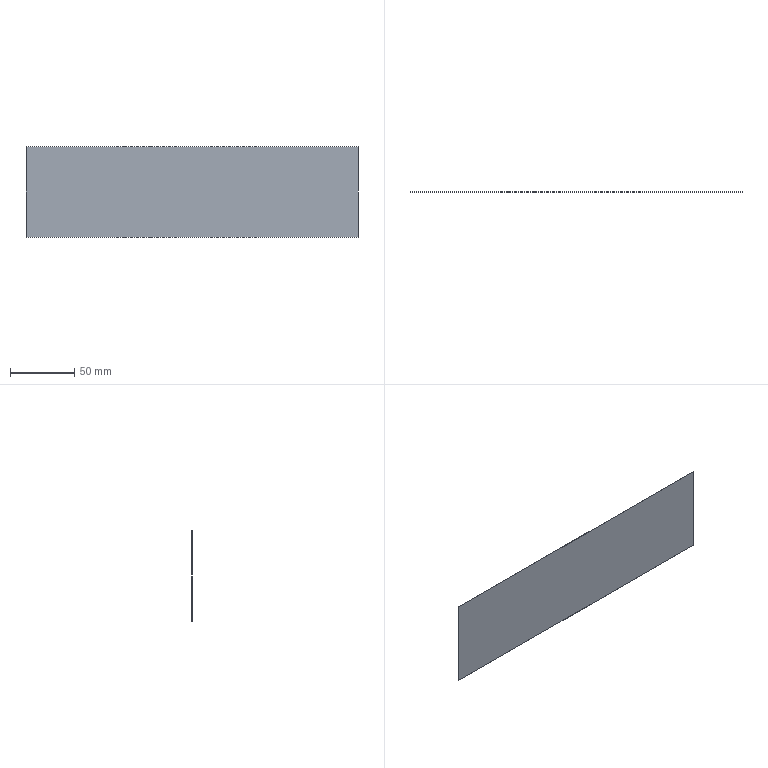Part | NX | features BREP 1 | 1 solid | 6 faces | box 258 x 0.1 x 70 mm | volume 1806 mm3 | plane 6
STEP:
#1=CARTESIAN_POINT('',(129.,0.,35.));
#2=VERTEX_POINT('',#1);
#3=CARTESIAN_POINT('',(129.,0.,-35.));
#4=VERTEX_POINT('',#3);
#5=CARTESIAN_POINT('',(129.,0.,-35.));
#6=DIRECTION('',(0.,0.,-1.));
#7=VECTOR('',#6,1000.);
#8=LINE('',#5,#7);
#9=EDGE_CURVE('',#2,#4,#8,.T.);
#10=ORIENTED_EDGE('',*,*,#9,.F.);
#11=CARTESIAN_POINT('',(-129.,0.,35.));
#12=VERTEX_POINT('',#11);
#13=CARTESIAN_POINT('',(-129.,0.,35.));
#14=DIRECTION('',(1.,0.,0.));
#15=VECTOR('',#14,1000.);
#16=LINE('',#13,#15);
#17=EDGE_CURVE('',#12,#2,#16,.T.);
#18=ORIENTED_EDGE('',*,*,#17,.F.);
#19=CARTESIAN_POINT('',(-129.,0.,-35.));
#20=VERTEX_POINT('',#19);
#21=CARTESIAN_POINT('',(-129.,0.,-35.));
#22=DIRECTION('',(0.,0.,1.));
#23=VECTOR('',#22,1000.);
#24=LINE('',#21,#23);
#25=EDGE_CURVE('',#20,#12,#24,.T.);
#26=ORIENTED_EDGE('',*,*,#25,.F.);
#27=CARTESIAN_POINT('',(-129.,0.,-35.));
#28=DIRECTION('',(-1.,0.,0.));
#29=VECTOR('',#28,1000.);
#30=LINE('',#27,#29);
#31=EDGE_CURVE('',#4,#20,#30,.T.);
#32=ORIENTED_EDGE('',*,*,#31,.F.);
#33=EDGE_LOOP('',(#10,#18,#26,#32));
#34=FACE_BOUND('',#33,.T.);
#35=CARTESIAN_POINT('',(0.,0.,0.));
#36=DIRECTION('',(0.,1.,0.));
#37=DIRECTION('',(0.,0.,1.));
#38=AXIS2_PLACEMENT_3D('',#35,#36,#37);
#39=PLANE('',#38);
#40=ADVANCED_FACE('',(#34),#39,.F.);
#41=CARTESIAN_POINT('',(129.,0.1,35.));
#42=VERTEX_POINT('',#41);
#43=CARTESIAN_POINT('',(129.,0.1,-35.));
#44=VERTEX_POINT('',#43);
#45=CARTESIAN_POINT('',(129.,0.1,-35.));
#46=DIRECTION('',(0.,0.,-1.));
#47=VECTOR('',#46,1000.);
#48=LINE('',#45,#47);
#49=EDGE_CURVE('',#42,#44,#48,.T.);
#50=ORIENTED_EDGE('',*,*,#49,.T.);
#51=CARTESIAN_POINT('',(-129.,0.1,-35.));
#52=VERTEX_POINT('',#51);
#53=CARTESIAN_POINT('',(-129.,0.1,-35.));
#54=DIRECTION('',(-1.,0.,0.));
#55=VECTOR('',#54,1000.);
#56=LINE('',#53,#55);
#57=EDGE_CURVE('',#44,#52,#56,.T.);
#58=ORIENTED_EDGE('',*,*,#57,.T.);
#59=CARTESIAN_POINT('',(-129.,0.1,35.));
#60=VERTEX_POINT('',#59);
#61=CARTESIAN_POINT('',(-129.,0.1,-35.));
#62=DIRECTION('',(0.,0.,1.));
#63=VECTOR('',#62,1000.);
#64=LINE('',#61,#63);
#65=EDGE_CURVE('',#52,#60,#64,.T.);
#66=ORIENTED_EDGE('',*,*,#65,.T.);
#67=CARTESIAN_POINT('',(-129.,0.1,35.));
#68=DIRECTION('',(1.,0.,0.));
#69=VECTOR('',#68,1000.);
#70=LINE('',#67,#69);
#71=EDGE_CURVE('',#60,#42,#70,.T.);
#72=ORIENTED_EDGE('',*,*,#71,.T.);
#73=EDGE_LOOP('',(#50,#58,#66,#72));
#74=FACE_BOUND('',#73,.T.);
#75=CARTESIAN_POINT('',(0.,0.1,0.));
#76=DIRECTION('',(0.,1.,0.));
#77=DIRECTION('',(0.,0.,1.));
#78=AXIS2_PLACEMENT_3D('',#75,#76,#77);
#79=PLANE('',#78);
#80=ADVANCED_FACE('',(#74),#79,.T.);
#81=ORIENTED_EDGE('',*,*,#17,.T.);
#82=CARTESIAN_POINT('',(129.,0.1,35.));
#83=DIRECTION('',(0.,-1.,0.));
#84=VECTOR('',#83,1000.);
#85=LINE('',#82,#84);
#86=EDGE_CURVE('',#42,#2,#85,.T.);
#87=ORIENTED_EDGE('',*,*,#86,.F.);
#88=ORIENTED_EDGE('',*,*,#71,.F.);
#89=CARTESIAN_POINT('',(-129.,0.1,35.));
#90=DIRECTION('',(0.,-1.,0.));
#91=VECTOR('',#90,1000.);
#92=LINE('',#89,#91);
#93=EDGE_CURVE('',#60,#12,#92,.T.);
#94=ORIENTED_EDGE('',*,*,#93,.T.);
#95=EDGE_LOOP('',(#81,#87,#88,#94));
#96=FACE_BOUND('',#95,.T.);
#97=CARTESIAN_POINT('',(-129.,0.1,35.));
#98=DIRECTION('',(0.,0.,-1.));
#99=DIRECTION('',(-1.,0.,0.));
#100=AXIS2_PLACEMENT_3D('',#97,#98,#99);
#101=PLANE('',#100);
#102=ADVANCED_FACE('',(#96),#101,.F.);
#103=ORIENTED_EDGE('',*,*,#25,.T.);
#104=ORIENTED_EDGE('',*,*,#93,.F.);
#105=ORIENTED_EDGE('',*,*,#65,.F.);
#106=CARTESIAN_POINT('',(-129.,0.1,-35.));
#107=DIRECTION('',(0.,-1.,0.));
#108=VECTOR('',#107,1000.);
#109=LINE('',#106,#108);
#110=EDGE_CURVE('',#52,#20,#109,.T.);
#111=ORIENTED_EDGE('',*,*,#110,.T.);
#112=EDGE_LOOP('',(#103,#104,#105,#111));
#113=FACE_BOUND('',#112,.T.);
#114=CARTESIAN_POINT('',(-129.,0.1,-35.));
#115=DIRECTION('',(1.,0.,0.));
#116=DIRECTION('',(0.,0.,-1.));
#117=AXIS2_PLACEMENT_3D('',#114,#115,#116);
#118=PLANE('',#117);
#119=ADVANCED_FACE('',(#113),#118,.F.);
#120=ORIENTED_EDGE('',*,*,#31,.T.);
#121=ORIENTED_EDGE('',*,*,#110,.F.);
#122=ORIENTED_EDGE('',*,*,#57,.F.);
#123=CARTESIAN_POINT('',(129.,0.1,-35.));
#124=DIRECTION('',(0.,-1.,0.));
#125=VECTOR('',#124,1000.);
#126=LINE('',#123,#125);
#127=EDGE_CURVE('',#44,#4,#126,.T.);
#128=ORIENTED_EDGE('',*,*,#127,.T.);
#129=EDGE_LOOP('',(#120,#121,#122,#128));
#130=FACE_BOUND('',#129,.T.);
#131=CARTESIAN_POINT('',(-129.,0.1,-35.));
#132=DIRECTION('',(0.,0.,1.));
#133=DIRECTION('',(1.,0.,0.));
#134=AXIS2_PLACEMENT_3D('',#131,#132,#133);
#135=PLANE('',#134);
#136=ADVANCED_FACE('',(#130),#135,.F.);
#137=ORIENTED_EDGE('',*,*,#9,.T.);
#138=ORIENTED_EDGE('',*,*,#127,.F.);
#139=ORIENTED_EDGE('',*,*,#49,.F.);
#140=ORIENTED_EDGE('',*,*,#86,.T.);
#141=EDGE_LOOP('',(#137,#138,#139,#140));
#142=FACE_BOUND('',#141,.T.);
#143=CARTESIAN_POINT('',(129.,0.1,-35.));
#144=DIRECTION('',(-1.,0.,0.));
#145=DIRECTION('',(0.,0.,1.));
#146=AXIS2_PLACEMENT_3D('',#143,#144,#145);
#147=PLANE('',#146);
#148=ADVANCED_FACE('',(#142),#147,.F.);
#149=CLOSED_SHELL('',(#40,#80,#102,#119,#136,#148));
#150=MANIFOLD_SOLID_BREP('',#149);
#151=(LENGTH_UNIT()NAMED_UNIT(*)SI_UNIT(.MILLI.,.METRE.));
#152=UNCERTAINTY_MEASURE_WITH_UNIT(LENGTH_MEASURE(0.00001),#151,'','');
#153=(NAMED_UNIT(*)PLANE_ANGLE_UNIT()SI_UNIT($,.RADIAN.));
#154=(NAMED_UNIT(*)SI_UNIT($,.STERADIAN.)SOLID_ANGLE_UNIT());
#155=(GEOMETRIC_REPRESENTATION_CONTEXT(3)GLOBAL_UNCERTAINTY_ASSIGNED_CONTEXT((#152))GLOBAL_UNIT_ASSIGNED_CONTEXT((#151,#153,#154))REPRESENTATION_CONTEXT('',''));
#156=ADVANCED_BREP_SHAPE_REPRESENTATION('',(#150),#155);